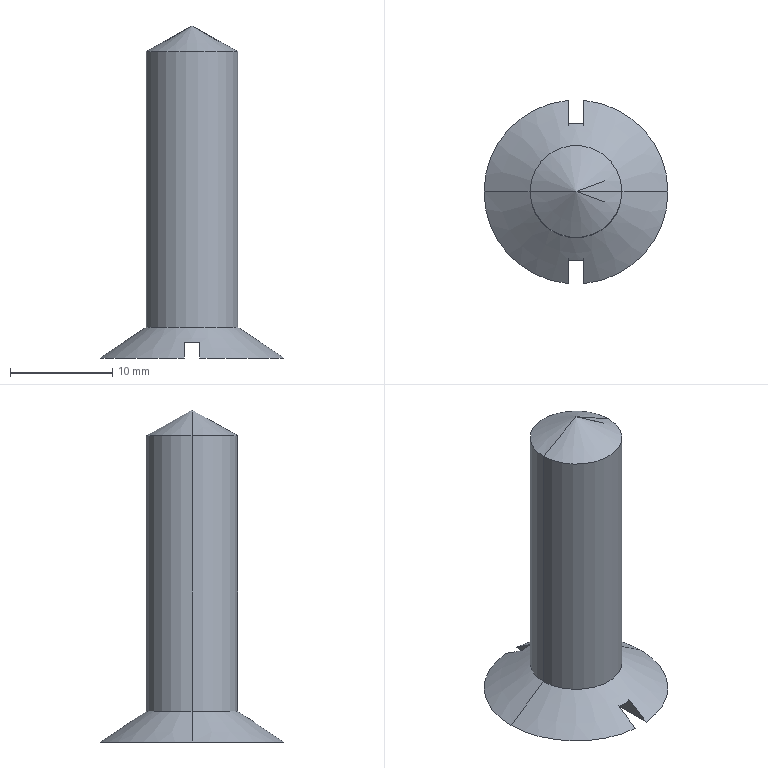Part | SolidWorks | features ICE 1, Revolution 1 | 1 solid | 11 faces | box 18 x 17.937 x 32.5 mm | volume 2181 mm3 | plane 5 | cone 4 | cylinder 2 | commonest cylinder face diameters 9 x2
STEP:
#1=CARTESIAN_POINT('',(-4.5,0.,-13.5));
#2=VERTEX_POINT('',#1);
#3=CARTESIAN_POINT('',(4.5,0.,-13.5));
#4=VERTEX_POINT('',#3);
#5=CARTESIAN_POINT('',(0.,0.,-13.5));
#6=DIRECTION('',(0.,0.,-1.));
#7=DIRECTION('',(-1.,0.,0.));
#8=AXIS2_PLACEMENT_3D('',#5,#6,#7);
#9=CIRCLE('',#8,4.5);
#10=EDGE_CURVE('',#2,#4,#9,.T.);
#11=ORIENTED_EDGE('',*,*,#10,.T.);
#12=CARTESIAN_POINT('',(9.,0.,-16.5));
#13=VERTEX_POINT('',#12);
#14=CARTESIAN_POINT('',(9.,0.,-16.5));
#15=DIRECTION('',(0.8321,0.,-0.5547));
#16=VECTOR('',#15,1000.);
#17=LINE('',#14,#16);
#18=EDGE_CURVE('',#4,#13,#17,.T.);
#19=ORIENTED_EDGE('',*,*,#18,.T.);
#20=CARTESIAN_POINT('',(0.75,8.969,-16.5));
#21=VERTEX_POINT('',#20);
#22=CARTESIAN_POINT('',(0.,0.,-16.5));
#23=DIRECTION('',(0.,0.,-1.));
#24=DIRECTION('',(-1.,0.,0.));
#25=AXIS2_PLACEMENT_3D('',#22,#23,#24);
#26=CIRCLE('',#25,9.);
#27=EDGE_CURVE('',#21,#13,#26,.T.);
#28=ORIENTED_EDGE('',*,*,#27,.F.);
#29=CARTESIAN_POINT('',(0.75,6.708,-15.));
#30=VERTEX_POINT('',#29);
#31=CARTESIAN_POINT('',(0.75,6.708,-15.));
#32=CARTESIAN_POINT('',(0.75,7.462,-15.499));
#33=CARTESIAN_POINT('',(0.75,8.215,-16.));
#34=CARTESIAN_POINT('',(0.75,8.969,-16.5));
#35=B_SPLINE_CURVE_WITH_KNOTS('',3,(#31,#32,#33,#34),.UNSPECIFIED.,.F.,.F.,(4,4),(0.03137,0.03405),.UNSPECIFIED.);
#36=EDGE_CURVE('',#30,#21,#35,.T.);
#37=ORIENTED_EDGE('',*,*,#36,.F.);
#38=CARTESIAN_POINT('',(-0.75,6.708,-15.));
#39=VERTEX_POINT('',#38);
#40=CARTESIAN_POINT('',(0.,0.,-15.));
#41=DIRECTION('',(0.,0.,-1.));
#42=DIRECTION('',(1.,0.,0.));
#43=AXIS2_PLACEMENT_3D('',#40,#41,#42);
#44=CIRCLE('',#43,6.75);
#45=EDGE_CURVE('',#39,#30,#44,.T.);
#46=ORIENTED_EDGE('',*,*,#45,.F.);
#47=CARTESIAN_POINT('',(-0.75,8.969,-16.5));
#48=VERTEX_POINT('',#47);
#49=CARTESIAN_POINT('',(-0.75,8.969,-16.5));
#50=CARTESIAN_POINT('',(-0.75,8.215,-16.));
#51=CARTESIAN_POINT('',(-0.75,7.462,-15.499));
#52=CARTESIAN_POINT('',(-0.75,6.708,-15.));
#53=B_SPLINE_CURVE_WITH_KNOTS('',3,(#49,#50,#51,#52),.UNSPECIFIED.,.F.,.F.,(4,4),(0.01306,0.01577),.UNSPECIFIED.);
#54=EDGE_CURVE('',#48,#39,#53,.T.);
#55=ORIENTED_EDGE('',*,*,#54,.F.);
#56=CARTESIAN_POINT('',(-9.,0.,-16.5));
#57=VERTEX_POINT('',#56);
#58=CARTESIAN_POINT('',(0.,0.,-16.5));
#59=DIRECTION('',(0.,0.,-1.));
#60=DIRECTION('',(-1.,0.,0.));
#61=AXIS2_PLACEMENT_3D('',#58,#59,#60);
#62=CIRCLE('',#61,9.);
#63=EDGE_CURVE('',#57,#48,#62,.T.);
#64=ORIENTED_EDGE('',*,*,#63,.F.);
#65=CARTESIAN_POINT('',(-9.,0.,-16.5));
#66=DIRECTION('',(-0.8321,0.,-0.5547));
#67=VECTOR('',#66,1000.);
#68=LINE('',#65,#67);
#69=EDGE_CURVE('',#2,#57,#68,.T.);
#70=ORIENTED_EDGE('',*,*,#69,.F.);
#71=EDGE_LOOP('',(#11,#19,#28,#37,#46,#55,#64,#70));
#72=FACE_OUTER_BOUND('',#71,.T.);
#73=CARTESIAN_POINT('',(0.,0.,-16.5));
#74=DIRECTION('',(0.,0.,-1.));
#75=DIRECTION('',(-1.,0.,0.));
#76=AXIS2_PLACEMENT_3D('',#73,#74,#75);
#77=CONICAL_SURFACE('',#76,9.,0.9828);
#78=ADVANCED_FACE('',(#72),#77,.T.);
#79=CARTESIAN_POINT('',(-4.5,0.,13.5));
#80=VERTEX_POINT('',#79);
#81=CARTESIAN_POINT('',(4.5,0.,13.5));
#82=VERTEX_POINT('',#81);
#83=CARTESIAN_POINT('',(0.,0.,13.5));
#84=DIRECTION('',(0.,0.,-1.));
#85=DIRECTION('',(-1.,0.,0.));
#86=AXIS2_PLACEMENT_3D('',#83,#84,#85);
#87=CIRCLE('',#86,4.5);
#88=EDGE_CURVE('',#80,#82,#87,.T.);
#89=ORIENTED_EDGE('',*,*,#88,.T.);
#90=CARTESIAN_POINT('',(4.5,0.,-13.5));
#91=DIRECTION('',(0.,0.,-1.));
#92=VECTOR('',#91,1000.);
#93=LINE('',#90,#92);
#94=EDGE_CURVE('',#82,#4,#93,.T.);
#95=ORIENTED_EDGE('',*,*,#94,.T.);
#96=ORIENTED_EDGE('',*,*,#10,.F.);
#97=CARTESIAN_POINT('',(-4.5,0.,-13.5));
#98=DIRECTION('',(0.,0.,-1.));
#99=VECTOR('',#98,1000.);
#100=LINE('',#97,#99);
#101=EDGE_CURVE('',#80,#2,#100,.T.);
#102=ORIENTED_EDGE('',*,*,#101,.F.);
#103=EDGE_LOOP('',(#89,#95,#96,#102));
#104=FACE_OUTER_BOUND('',#103,.T.);
#105=CARTESIAN_POINT('',(0.,0.,-13.5));
#106=DIRECTION('',(0.,0.,-1.));
#107=DIRECTION('',(-1.,0.,0.));
#108=AXIS2_PLACEMENT_3D('',#105,#106,#107);
#109=CYLINDRICAL_SURFACE('',#108,4.5);
#110=ADVANCED_FACE('',(#104),#109,.T.);
#111=CARTESIAN_POINT('',(0.,0.,16.));
#112=VERTEX_POINT('',#111);
#113=CARTESIAN_POINT('',(-4.5,0.,13.5));
#114=DIRECTION('',(-0.8742,0.,-0.4856));
#115=VECTOR('',#114,1000.);
#116=LINE('',#113,#115);
#117=EDGE_CURVE('',#112,#80,#116,.T.);
#118=ORIENTED_EDGE('',*,*,#117,.F.);
#119=CARTESIAN_POINT('',(4.5,0.,13.5));
#120=DIRECTION('',(0.8742,0.,-0.4856));
#121=VECTOR('',#120,1000.);
#122=LINE('',#119,#121);
#123=EDGE_CURVE('',#112,#82,#122,.T.);
#124=ORIENTED_EDGE('',*,*,#123,.T.);
#125=ORIENTED_EDGE('',*,*,#88,.F.);
#126=EDGE_LOOP('',(#118,#124,#125));
#127=FACE_OUTER_BOUND('',#126,.T.);
#128=CARTESIAN_POINT('',(0.,0.,13.5));
#129=DIRECTION('',(0.,0.,-1.));
#130=DIRECTION('',(-1.,0.,0.));
#131=AXIS2_PLACEMENT_3D('',#128,#129,#130);
#132=CONICAL_SURFACE('',#131,4.5,1.064);
#133=ADVANCED_FACE('',(#127),#132,.T.);
#134=CARTESIAN_POINT('',(0.75,-8.969,-16.5));
#135=VERTEX_POINT('',#134);
#136=CARTESIAN_POINT('',(0.75,0.,-16.5));
#137=DIRECTION('',(0.,-1.,0.));
#138=VECTOR('',#137,1000.);
#139=LINE('',#136,#138);
#140=EDGE_CURVE('',#21,#135,#139,.T.);
#141=ORIENTED_EDGE('',*,*,#140,.F.);
#142=ORIENTED_EDGE('',*,*,#27,.T.);
#143=CARTESIAN_POINT('',(0.,0.,-16.5));
#144=DIRECTION('',(0.,0.,-1.));
#145=DIRECTION('',(-1.,0.,0.));
#146=AXIS2_PLACEMENT_3D('',#143,#144,#145);
#147=CIRCLE('',#146,9.);
#148=EDGE_CURVE('',#13,#135,#147,.T.);
#149=ORIENTED_EDGE('',*,*,#148,.T.);
#150=EDGE_LOOP('',(#141,#142,#149));
#151=FACE_OUTER_BOUND('',#150,.T.);
#152=CARTESIAN_POINT('',(0.,0.,-16.5));
#153=DIRECTION('',(0.,0.,-1.));
#154=DIRECTION('',(-1.,0.,0.));
#155=AXIS2_PLACEMENT_3D('',#152,#153,#154);
#156=PLANE('',#155);
#157=ADVANCED_FACE('',(#151),#156,.T.);
#158=ORIENTED_EDGE('',*,*,#123,.F.);
#159=ORIENTED_EDGE('',*,*,#117,.T.);
#160=CARTESIAN_POINT('',(0.,0.,13.5));
#161=DIRECTION('',(0.,0.,-1.));
#162=DIRECTION('',(-1.,0.,0.));
#163=AXIS2_PLACEMENT_3D('',#160,#161,#162);
#164=CIRCLE('',#163,4.5);
#165=EDGE_CURVE('',#82,#80,#164,.T.);
#166=ORIENTED_EDGE('',*,*,#165,.F.);
#167=EDGE_LOOP('',(#158,#159,#166));
#168=FACE_OUTER_BOUND('',#167,.T.);
#169=CARTESIAN_POINT('',(0.,0.,13.5));
#170=DIRECTION('',(0.,0.,-1.));
#171=DIRECTION('',(-1.,0.,0.));
#172=AXIS2_PLACEMENT_3D('',#169,#170,#171);
#173=CONICAL_SURFACE('',#172,4.5,1.064);
#174=ADVANCED_FACE('',(#168),#173,.T.);
#175=ORIENTED_EDGE('',*,*,#94,.F.);
#176=ORIENTED_EDGE('',*,*,#165,.T.);
#177=ORIENTED_EDGE('',*,*,#101,.T.);
#178=CARTESIAN_POINT('',(0.,0.,-13.5));
#179=DIRECTION('',(0.,0.,-1.));
#180=DIRECTION('',(-1.,0.,0.));
#181=AXIS2_PLACEMENT_3D('',#178,#179,#180);
#182=CIRCLE('',#181,4.5);
#183=EDGE_CURVE('',#4,#2,#182,.T.);
#184=ORIENTED_EDGE('',*,*,#183,.F.);
#185=EDGE_LOOP('',(#175,#176,#177,#184));
#186=FACE_OUTER_BOUND('',#185,.T.);
#187=CARTESIAN_POINT('',(0.,0.,-13.5));
#188=DIRECTION('',(0.,0.,-1.));
#189=DIRECTION('',(-1.,0.,0.));
#190=AXIS2_PLACEMENT_3D('',#187,#188,#189);
#191=CYLINDRICAL_SURFACE('',#190,4.5);
#192=ADVANCED_FACE('',(#186),#191,.T.);
#193=ORIENTED_EDGE('',*,*,#18,.F.);
#194=ORIENTED_EDGE('',*,*,#183,.T.);
#195=ORIENTED_EDGE('',*,*,#69,.T.);
#196=CARTESIAN_POINT('',(-0.75,-8.969,-16.5));
#197=VERTEX_POINT('',#196);
#198=CARTESIAN_POINT('',(0.,0.,-16.5));
#199=DIRECTION('',(0.,0.,-1.));
#200=DIRECTION('',(-1.,0.,0.));
#201=AXIS2_PLACEMENT_3D('',#198,#199,#200);
#202=CIRCLE('',#201,9.);
#203=EDGE_CURVE('',#197,#57,#202,.T.);
#204=ORIENTED_EDGE('',*,*,#203,.F.);
#205=CARTESIAN_POINT('',(-0.75,-6.708,-15.));
#206=VERTEX_POINT('',#205);
#207=CARTESIAN_POINT('',(-0.75,-6.708,-15.));
#208=CARTESIAN_POINT('',(-0.75,-7.462,-15.499));
#209=CARTESIAN_POINT('',(-0.75,-8.215,-16.));
#210=CARTESIAN_POINT('',(-0.75,-8.969,-16.5));
#211=B_SPLINE_CURVE_WITH_KNOTS('',3,(#207,#208,#209,#210),.UNSPECIFIED.,.F.,.F.,(4,4),(0.03137,0.03405),.UNSPECIFIED.);
#212=EDGE_CURVE('',#206,#197,#211,.T.);
#213=ORIENTED_EDGE('',*,*,#212,.F.);
#214=CARTESIAN_POINT('',(0.75,-6.708,-15.));
#215=VERTEX_POINT('',#214);
#216=CARTESIAN_POINT('',(0.,0.,-15.));
#217=DIRECTION('',(0.,0.,-1.));
#218=DIRECTION('',(1.,0.,0.));
#219=AXIS2_PLACEMENT_3D('',#216,#217,#218);
#220=CIRCLE('',#219,6.75);
#221=EDGE_CURVE('',#215,#206,#220,.T.);
#222=ORIENTED_EDGE('',*,*,#221,.F.);
#223=CARTESIAN_POINT('',(0.75,-8.969,-16.5));
#224=CARTESIAN_POINT('',(0.75,-8.215,-16.));
#225=CARTESIAN_POINT('',(0.75,-7.462,-15.499));
#226=CARTESIAN_POINT('',(0.75,-6.708,-15.));
#227=B_SPLINE_CURVE_WITH_KNOTS('',3,(#223,#224,#225,#226),.UNSPECIFIED.,.F.,.F.,(4,4),(0.01306,0.01577),.UNSPECIFIED.);
#228=EDGE_CURVE('',#135,#215,#227,.T.);
#229=ORIENTED_EDGE('',*,*,#228,.F.);
#230=ORIENTED_EDGE('',*,*,#148,.F.);
#231=EDGE_LOOP('',(#193,#194,#195,#204,#213,#222,#229,#230));
#232=FACE_OUTER_BOUND('',#231,.T.);
#233=CARTESIAN_POINT('',(0.,0.,-16.5));
#234=DIRECTION('',(0.,0.,-1.));
#235=DIRECTION('',(-1.,0.,0.));
#236=AXIS2_PLACEMENT_3D('',#233,#234,#235);
#237=CONICAL_SURFACE('',#236,9.,0.9828);
#238=ADVANCED_FACE('',(#232),#237,.T.);
#239=CARTESIAN_POINT('',(-0.75,0.,-16.5));
#240=DIRECTION('',(0.,1.,0.));
#241=VECTOR('',#240,1000.);
#242=LINE('',#239,#241);
#243=EDGE_CURVE('',#197,#48,#242,.T.);
#244=ORIENTED_EDGE('',*,*,#243,.F.);
#245=ORIENTED_EDGE('',*,*,#203,.T.);
#246=ORIENTED_EDGE('',*,*,#63,.T.);
#247=EDGE_LOOP('',(#244,#245,#246));
#248=FACE_OUTER_BOUND('',#247,.T.);
#249=CARTESIAN_POINT('',(0.,0.,-16.5));
#250=DIRECTION('',(0.,0.,-1.));
#251=DIRECTION('',(-1.,0.,0.));
#252=AXIS2_PLACEMENT_3D('',#249,#250,#251);
#253=PLANE('',#252);
#254=ADVANCED_FACE('',(#248),#253,.T.);
#255=ORIENTED_EDGE('',*,*,#228,.T.);
#256=CARTESIAN_POINT('',(0.75,-15.,-15.));
#257=DIRECTION('',(0.,1.,0.));
#258=VECTOR('',#257,1000.);
#259=LINE('',#256,#258);
#260=EDGE_CURVE('',#215,#30,#259,.T.);
#261=ORIENTED_EDGE('',*,*,#260,.T.);
#262=ORIENTED_EDGE('',*,*,#36,.T.);
#263=ORIENTED_EDGE('',*,*,#140,.T.);
#264=EDGE_LOOP('',(#255,#261,#262,#263));
#265=FACE_OUTER_BOUND('',#264,.T.);
#266=CARTESIAN_POINT('',(0.75,-15.,-16.5));
#267=DIRECTION('',(1.,0.,0.));
#268=DIRECTION('',(0.,0.,-1.));
#269=AXIS2_PLACEMENT_3D('',#266,#267,#268);
#270=PLANE('',#269);
#271=ADVANCED_FACE('',(#265),#270,.F.);
#272=ORIENTED_EDGE('',*,*,#221,.T.);
#273=CARTESIAN_POINT('',(-0.75,-15.,-15.));
#274=DIRECTION('',(0.,1.,0.));
#275=VECTOR('',#274,1000.);
#276=LINE('',#273,#275);
#277=EDGE_CURVE('',#206,#39,#276,.T.);
#278=ORIENTED_EDGE('',*,*,#277,.T.);
#279=ORIENTED_EDGE('',*,*,#45,.T.);
#280=ORIENTED_EDGE('',*,*,#260,.F.);
#281=EDGE_LOOP('',(#272,#278,#279,#280));
#282=FACE_OUTER_BOUND('',#281,.T.);
#283=CARTESIAN_POINT('',(-0.75,-15.,-15.));
#284=DIRECTION('',(0.,0.,1.));
#285=DIRECTION('',(1.,0.,0.));
#286=AXIS2_PLACEMENT_3D('',#283,#284,#285);
#287=PLANE('',#286);
#288=ADVANCED_FACE('',(#282),#287,.F.);
#289=ORIENTED_EDGE('',*,*,#54,.T.);
#290=ORIENTED_EDGE('',*,*,#277,.F.);
#291=ORIENTED_EDGE('',*,*,#212,.T.);
#292=ORIENTED_EDGE('',*,*,#243,.T.);
#293=EDGE_LOOP('',(#289,#290,#291,#292));
#294=FACE_OUTER_BOUND('',#293,.T.);
#295=CARTESIAN_POINT('',(-0.75,-15.,-15.));
#296=DIRECTION('',(-1.,0.,0.));
#297=DIRECTION('',(0.,0.,1.));
#298=AXIS2_PLACEMENT_3D('',#295,#296,#297);
#299=PLANE('',#298);
#300=ADVANCED_FACE('',(#294),#299,.F.);
#301=CLOSED_SHELL('',(#78,#110,#133,#157,#174,#192,#238,#254,#271,#288,#300));
#302=MANIFOLD_SOLID_BREP('',#301);
#303=CARTESIAN_POINT('',(0.,0.,0.));
#304=DIRECTION('',(0.,0.,1.));
#305=DIRECTION('',(1.,0.,0.));
#306=AXIS2_PLACEMENT_3D('',#303,#304,#305);
#307=(LENGTH_UNIT()NAMED_UNIT(*)SI_UNIT(.MILLI.,.METRE.));
#308=UNCERTAINTY_MEASURE_WITH_UNIT(LENGTH_MEASURE(0.00001),#307,'','');
#309=(NAMED_UNIT(*)PLANE_ANGLE_UNIT()SI_UNIT($,.RADIAN.));
#310=(NAMED_UNIT(*)SI_UNIT($,.STERADIAN.)SOLID_ANGLE_UNIT());
#311=(GEOMETRIC_REPRESENTATION_CONTEXT(3)GLOBAL_UNCERTAINTY_ASSIGNED_CONTEXT((#308))GLOBAL_UNIT_ASSIGNED_CONTEXT((#307,#309,#310))REPRESENTATION_CONTEXT('',''));
#312=ADVANCED_BREP_SHAPE_REPRESENTATION('',(#302,#306),#311);